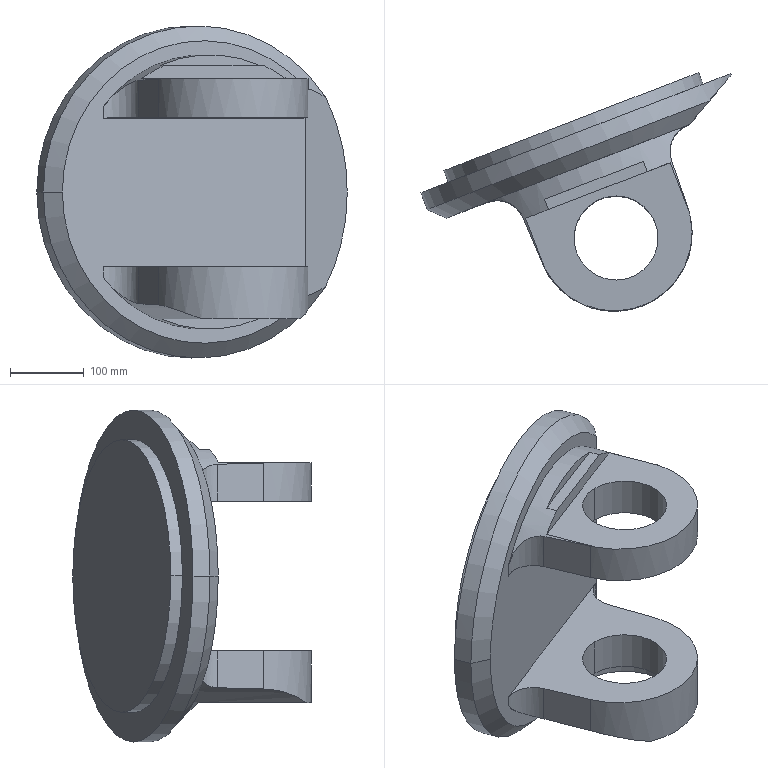Part | SolidWorks | features ICE 3, MoveFace 2, BaseBody 1, Chamfer 1, Scale 1 | 1 solid | 38 faces | box 420.674 x 323.225 x 450 mm | volume 11948863 mm3 | cylinder 19 | plane 17 | cone 2 | commonest cylinder face diameters 75.6 x4 114 x4 141.6 x2 211.33 x2 370 x2 372 x2